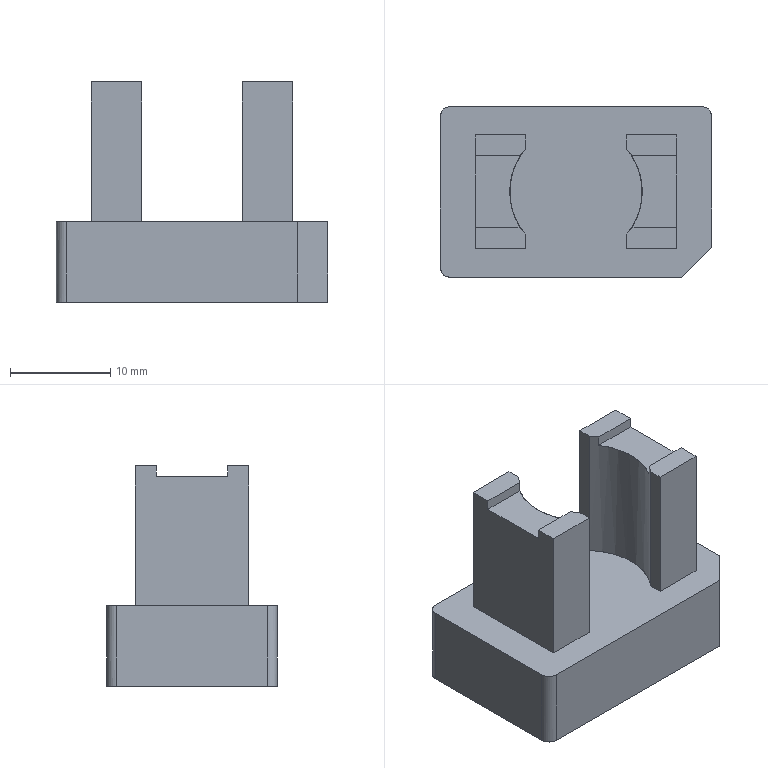CAM job | PowerMill | 3-axis milling, other | part box 27 x 17 x 21.929 mm
Tools:
number,name,type,diameter,tip_radius,length,cutting_length,overhang,flutes,holder,toolpaths_using
1,D10C,end_mill,10.0,0.0,60.0,,30.0,1,D42L35,1
1,D10C_1_1_1,end_mill,10.0,0.0,60.0,,22.36,1,D42L35,3
2,D4C_1_1,end_mill,4.0,0.0,30.0,,14.12,1,D42L35,1
3,D10_1_1_1,end_mill,10.0,0.0,60.0,,22.08,1,D42L35,3
14,D4_1_1,end_mill,4.0,0.0,30.0,,14.08,1,D42L35,2
13,Text_D4_1_1,taper_spherical,4.0,0.3,60.0,,14.2,1,D42L35,1
Operations:
program,toolpath,strategy,tool,tool_number,tool_diameter,tip_radius,flutes,spindle_rpm,feed_cut,surface_speed_m_min_computed,feed_per_tooth_computed,tolerance,thickness,stepover,stepdown,cut_length,cut_time_min,total_time_min,workplane
26-S-2-F,精公开粗01-扫面平行-D10C,raster_area_clear,D10C_1_1_1,1,10.0,0.0,1.0,8000.0,10000.0,251.33,1.25,0.03,0.28,6.0,1.0,185.36,0.018,0.0241,
26-S-2-F,精公开粗01-外形偏置-D10C,offset_area_clear,D10C_1_1_1,1,10.0,0.0,1.0,8000.0,10000.0,251.33,1.25,0.03,0.28,6.0,1.0,7998.838,0.8,0.8873,
26-S-2-F,精公开粗01-基准台等高-D10C,constantz,D10C_1_1_1,1,10.0,0.0,1.0,8000.0,10000.0,251.33,1.25,0.03,0.07,5.0,0.4,2569.108,0.257,0.2667,
26-S-2-F,精公再粗02-外形偏置-D4C,offset_area_clear,D4C_1_1,2,4.0,0.0,1.0,18000.0,6000.0,226.19,0.3333,0.03,0.0,2.0,1.0,9039.041,1.506,2.239,
26-S-2-F,精公基准台01-平坦面平行-D10,raster_area_clear,D10_1_1_1,3,10.0,0.0,1.0,8500.0,600.0,267.04,0.0706,0.005,0.38,5.0,1.0,165.234,0.275,0.367,
26-S-2-F,精公基准台01-基准面偏置-D10,offset_area_clear,D10_1_1_1,3,10.0,0.0,1.0,8500.0,600.0,267.04,0.0706,0.005,0.38,5.0,1.0,107.163,0.179,0.1979,
26-S-2-F,精公基准台01-基准台侧光-D10,profile_area_clear,D10_1_1_1,3,10.0,0.0,1.0,8500.0,600.0,267.04,0.0706,0.005,0.0,0.08,1.0,233.233,0.389,0.4532,
26-S-2-F,精公精光01-等高-D4,constantz,D4_1_1,14,4.0,0.0,1.0,18000.0,2000.0,226.19,0.1111,0.005,-0.075,5.0,0.07,18440.623,9.22,9.243,
26-S-2-F,精公精光01-笔式-D4,pencil_corner,D4_1_1,14,4.0,0.0,1.0,18000.0,600.0,226.19,0.0333,0.005,-0.075,5.0,1.0,37.138,0.062,0.095,
26-S-2-F,精公刻字01-刻字-Text_D4,pattern,Text_D4_1_1,13,4.0,0.3,1.0,15000.0,1000.0,188.5,0.0667,0.005,0.0,5.0,1.0,27.859,0.028,0.0428,
,精公开粗01-外形偏置-D10C_Reference,offset_area_clear,D10C,1,10.0,0.0,1.0,8000.0,10000.0,251.33,1.25,0.03,0.28,6.0,1.0,15975.975,1.598,1.77,